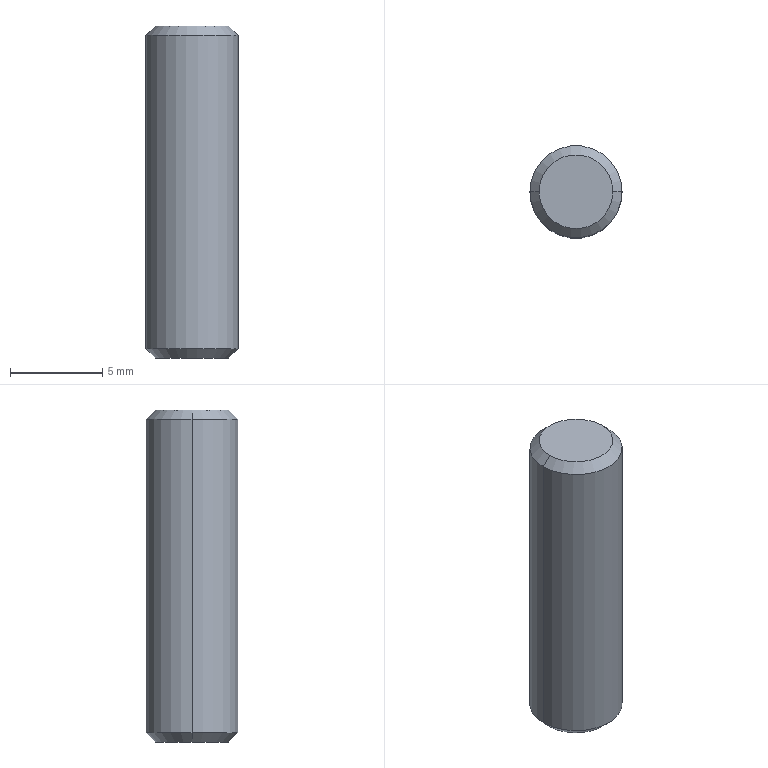Part | STEP file | Needle roller domestic φ5-18-1 | 1 solid | 8 faces | box 5 x 5 x 18 mm | volume 349.764 mm3 | cone 4 | cylinder 2 | plane 2 | commonest cylinder face diameters 5 x2
STEP:
#1=CARTESIAN_POINT('',(-2.,0.,0.));
#2=VERTEX_POINT('',#1);
#3=CARTESIAN_POINT('',(2.,0.,0.));
#4=VERTEX_POINT('',#3);
#5=CARTESIAN_POINT('',(0.,0.,0.));
#6=DIRECTION('',(0.,0.,-1.));
#7=DIRECTION('',(1.,0.,0.));
#8=AXIS2_PLACEMENT_3D('',#5,#6,#7);
#9=CIRCLE('',#8,2.);
#10=EDGE_CURVE('',#2,#4,#9,.T.);
#11=ORIENTED_EDGE('',*,*,#10,.F.);
#12=CARTESIAN_POINT('',(-2.5,0.,0.5));
#13=VERTEX_POINT('',#12);
#14=CARTESIAN_POINT('',(-2.5,0.,0.5));
#15=DIRECTION('',(-0.7071,0.,0.7071));
#16=VECTOR('',#15,1000.);
#17=LINE('',#14,#16);
#18=EDGE_CURVE('',#2,#13,#17,.T.);
#19=ORIENTED_EDGE('',*,*,#18,.T.);
#20=CARTESIAN_POINT('',(2.5,0.,0.5));
#21=VERTEX_POINT('',#20);
#22=CARTESIAN_POINT('',(0.,0.,0.5));
#23=DIRECTION('',(0.,0.,1.));
#24=DIRECTION('',(1.,0.,0.));
#25=AXIS2_PLACEMENT_3D('',#22,#23,#24);
#26=CIRCLE('',#25,2.5);
#27=EDGE_CURVE('',#21,#13,#26,.T.);
#28=ORIENTED_EDGE('',*,*,#27,.F.);
#29=CARTESIAN_POINT('',(2.5,0.,0.5));
#30=DIRECTION('',(0.7071,0.,0.7071));
#31=VECTOR('',#30,1000.);
#32=LINE('',#29,#31);
#33=EDGE_CURVE('',#4,#21,#32,.T.);
#34=ORIENTED_EDGE('',*,*,#33,.F.);
#35=EDGE_LOOP('',(#11,#19,#28,#34));
#36=FACE_OUTER_BOUND('',#35,.T.);
#37=CARTESIAN_POINT('',(0.,0.,0.5));
#38=DIRECTION('',(0.,0.,1.));
#39=DIRECTION('',(1.,0.,0.));
#40=AXIS2_PLACEMENT_3D('',#37,#38,#39);
#41=CONICAL_SURFACE('',#40,2.5,0.7854);
#42=ADVANCED_FACE('',(#36),#41,.T.);
#43=CARTESIAN_POINT('',(2.,0.,18.));
#44=VERTEX_POINT('',#43);
#45=CARTESIAN_POINT('',(-2.,0.,18.));
#46=VERTEX_POINT('',#45);
#47=CARTESIAN_POINT('',(0.,0.,18.));
#48=DIRECTION('',(0.,0.,1.));
#49=DIRECTION('',(1.,0.,0.));
#50=AXIS2_PLACEMENT_3D('',#47,#48,#49);
#51=CIRCLE('',#50,2.);
#52=EDGE_CURVE('',#44,#46,#51,.T.);
#53=ORIENTED_EDGE('',*,*,#52,.F.);
#54=CARTESIAN_POINT('',(2.5,0.,17.5));
#55=VERTEX_POINT('',#54);
#56=CARTESIAN_POINT('',(2.,0.,18.));
#57=DIRECTION('',(0.7071,0.,-0.7071));
#58=VECTOR('',#57,1000.);
#59=LINE('',#56,#58);
#60=EDGE_CURVE('',#44,#55,#59,.T.);
#61=ORIENTED_EDGE('',*,*,#60,.T.);
#62=CARTESIAN_POINT('',(-2.5,0.,17.5));
#63=VERTEX_POINT('',#62);
#64=CARTESIAN_POINT('',(0.,0.,17.5));
#65=DIRECTION('',(0.,0.,-1.));
#66=DIRECTION('',(1.,0.,0.));
#67=AXIS2_PLACEMENT_3D('',#64,#65,#66);
#68=CIRCLE('',#67,2.5);
#69=EDGE_CURVE('',#63,#55,#68,.T.);
#70=ORIENTED_EDGE('',*,*,#69,.F.);
#71=CARTESIAN_POINT('',(-2.,0.,18.));
#72=DIRECTION('',(-0.7071,0.,-0.7071));
#73=VECTOR('',#72,1000.);
#74=LINE('',#71,#73);
#75=EDGE_CURVE('',#46,#63,#74,.T.);
#76=ORIENTED_EDGE('',*,*,#75,.F.);
#77=EDGE_LOOP('',(#53,#61,#70,#76));
#78=FACE_OUTER_BOUND('',#77,.T.);
#79=CARTESIAN_POINT('',(0.,0.,18.));
#80=DIRECTION('',(0.,0.,-1.));
#81=DIRECTION('',(-1.,0.,0.));
#82=AXIS2_PLACEMENT_3D('',#79,#80,#81);
#83=CONICAL_SURFACE('',#82,2.,0.7854);
#84=ADVANCED_FACE('',(#78),#83,.T.);
#85=ORIENTED_EDGE('',*,*,#69,.T.);
#86=CARTESIAN_POINT('',(2.5,0.,18.));
#87=DIRECTION('',(0.,0.,-1.));
#88=VECTOR('',#87,1000.);
#89=LINE('',#86,#88);
#90=EDGE_CURVE('',#55,#21,#89,.T.);
#91=ORIENTED_EDGE('',*,*,#90,.T.);
#92=ORIENTED_EDGE('',*,*,#27,.T.);
#93=CARTESIAN_POINT('',(-2.5,0.,18.));
#94=DIRECTION('',(0.,0.,-1.));
#95=VECTOR('',#94,1000.);
#96=LINE('',#93,#95);
#97=EDGE_CURVE('',#63,#13,#96,.T.);
#98=ORIENTED_EDGE('',*,*,#97,.F.);
#99=EDGE_LOOP('',(#85,#91,#92,#98));
#100=FACE_OUTER_BOUND('',#99,.T.);
#101=CARTESIAN_POINT('',(0.,0.,18.));
#102=DIRECTION('',(0.,0.,-1.));
#103=DIRECTION('',(-1.,0.,0.));
#104=AXIS2_PLACEMENT_3D('',#101,#102,#103);
#105=CYLINDRICAL_SURFACE('',#104,2.5);
#106=ADVANCED_FACE('',(#100),#105,.T.);
#107=ORIENTED_EDGE('',*,*,#90,.F.);
#108=CARTESIAN_POINT('',(0.,0.,17.5));
#109=DIRECTION('',(0.,0.,-1.));
#110=DIRECTION('',(1.,0.,0.));
#111=AXIS2_PLACEMENT_3D('',#108,#109,#110);
#112=CIRCLE('',#111,2.5);
#113=EDGE_CURVE('',#55,#63,#112,.T.);
#114=ORIENTED_EDGE('',*,*,#113,.T.);
#115=ORIENTED_EDGE('',*,*,#97,.T.);
#116=CARTESIAN_POINT('',(0.,0.,0.5));
#117=DIRECTION('',(0.,0.,1.));
#118=DIRECTION('',(1.,0.,0.));
#119=AXIS2_PLACEMENT_3D('',#116,#117,#118);
#120=CIRCLE('',#119,2.5);
#121=EDGE_CURVE('',#13,#21,#120,.T.);
#122=ORIENTED_EDGE('',*,*,#121,.T.);
#123=EDGE_LOOP('',(#107,#114,#115,#122));
#124=FACE_OUTER_BOUND('',#123,.T.);
#125=CARTESIAN_POINT('',(0.,0.,18.));
#126=DIRECTION('',(0.,0.,-1.));
#127=DIRECTION('',(-1.,0.,0.));
#128=AXIS2_PLACEMENT_3D('',#125,#126,#127);
#129=CYLINDRICAL_SURFACE('',#128,2.5);
#130=ADVANCED_FACE('',(#124),#129,.T.);
#131=CARTESIAN_POINT('',(0.,0.,18.));
#132=DIRECTION('',(0.,0.,1.));
#133=DIRECTION('',(1.,0.,0.));
#134=AXIS2_PLACEMENT_3D('',#131,#132,#133);
#135=CIRCLE('',#134,2.);
#136=EDGE_CURVE('',#46,#44,#135,.T.);
#137=ORIENTED_EDGE('',*,*,#136,.T.);
#138=ORIENTED_EDGE('',*,*,#52,.T.);
#139=EDGE_LOOP('',(#137,#138));
#140=FACE_OUTER_BOUND('',#139,.T.);
#141=CARTESIAN_POINT('',(0.,0.,18.));
#142=DIRECTION('',(0.,0.,1.));
#143=DIRECTION('',(1.,0.,0.));
#144=AXIS2_PLACEMENT_3D('',#141,#142,#143);
#145=PLANE('',#144);
#146=ADVANCED_FACE('',(#140),#145,.T.);
#147=CARTESIAN_POINT('',(0.,0.,0.));
#148=DIRECTION('',(0.,0.,-1.));
#149=DIRECTION('',(1.,0.,0.));
#150=AXIS2_PLACEMENT_3D('',#147,#148,#149);
#151=CIRCLE('',#150,2.);
#152=EDGE_CURVE('',#4,#2,#151,.T.);
#153=ORIENTED_EDGE('',*,*,#152,.T.);
#154=ORIENTED_EDGE('',*,*,#10,.T.);
#155=EDGE_LOOP('',(#153,#154));
#156=FACE_OUTER_BOUND('',#155,.T.);
#157=CARTESIAN_POINT('',(0.,0.,0.));
#158=DIRECTION('',(0.,0.,1.));
#159=DIRECTION('',(1.,0.,0.));
#160=AXIS2_PLACEMENT_3D('',#157,#158,#159);
#161=PLANE('',#160);
#162=ADVANCED_FACE('',(#156),#161,.F.);
#163=ORIENTED_EDGE('',*,*,#60,.F.);
#164=ORIENTED_EDGE('',*,*,#136,.F.);
#165=ORIENTED_EDGE('',*,*,#75,.T.);
#166=ORIENTED_EDGE('',*,*,#113,.F.);
#167=EDGE_LOOP('',(#163,#164,#165,#166));
#168=FACE_OUTER_BOUND('',#167,.T.);
#169=CARTESIAN_POINT('',(0.,0.,18.));
#170=DIRECTION('',(0.,0.,-1.));
#171=DIRECTION('',(-1.,0.,0.));
#172=AXIS2_PLACEMENT_3D('',#169,#170,#171);
#173=CONICAL_SURFACE('',#172,2.,0.7854);
#174=ADVANCED_FACE('',(#168),#173,.T.);
#175=ORIENTED_EDGE('',*,*,#18,.F.);
#176=ORIENTED_EDGE('',*,*,#152,.F.);
#177=ORIENTED_EDGE('',*,*,#33,.T.);
#178=ORIENTED_EDGE('',*,*,#121,.F.);
#179=EDGE_LOOP('',(#175,#176,#177,#178));
#180=FACE_OUTER_BOUND('',#179,.T.);
#181=CARTESIAN_POINT('',(0.,0.,0.5));
#182=DIRECTION('',(0.,0.,1.));
#183=DIRECTION('',(1.,0.,0.));
#184=AXIS2_PLACEMENT_3D('',#181,#182,#183);
#185=CONICAL_SURFACE('',#184,2.5,0.7854);
#186=ADVANCED_FACE('',(#180),#185,.T.);
#187=CLOSED_SHELL('',(#42,#84,#106,#130,#146,#162,#174,#186));
#188=MANIFOLD_SOLID_BREP('',#187);
#189=CARTESIAN_POINT('',(0.,0.,0.));
#190=DIRECTION('',(0.,0.,1.));
#191=DIRECTION('',(1.,0.,0.));
#192=AXIS2_PLACEMENT_3D('',#189,#190,#191);
#193=(LENGTH_UNIT()NAMED_UNIT(*)SI_UNIT(.MILLI.,.METRE.));
#194=UNCERTAINTY_MEASURE_WITH_UNIT(LENGTH_MEASURE(0.00001),#193,'','');
#195=(NAMED_UNIT(*)PLANE_ANGLE_UNIT()SI_UNIT($,.RADIAN.));
#196=(NAMED_UNIT(*)SI_UNIT($,.STERADIAN.)SOLID_ANGLE_UNIT());
#197=(GEOMETRIC_REPRESENTATION_CONTEXT(3)GLOBAL_UNCERTAINTY_ASSIGNED_CONTEXT((#194))GLOBAL_UNIT_ASSIGNED_CONTEXT((#193,#195,#196))REPRESENTATION_CONTEXT('',''));
#198=ADVANCED_BREP_SHAPE_REPRESENTATION('',(#188,#192),#197);